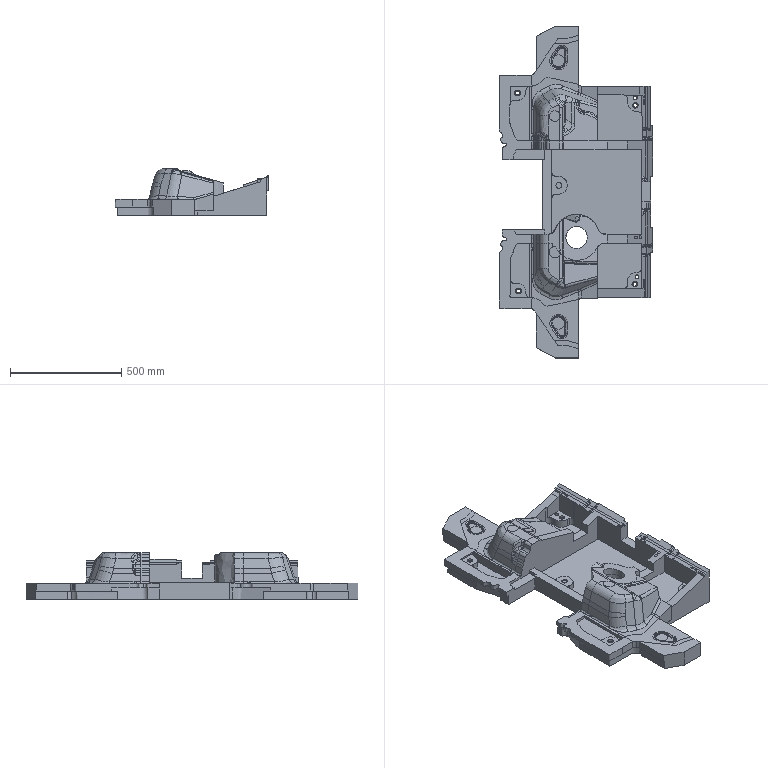Part | NX | features solid 2 | 1 solid | 558 faces | box 690.824 x 1490 x 210.501 mm | volume 61253517 mm3 | spline 536 | plane 22